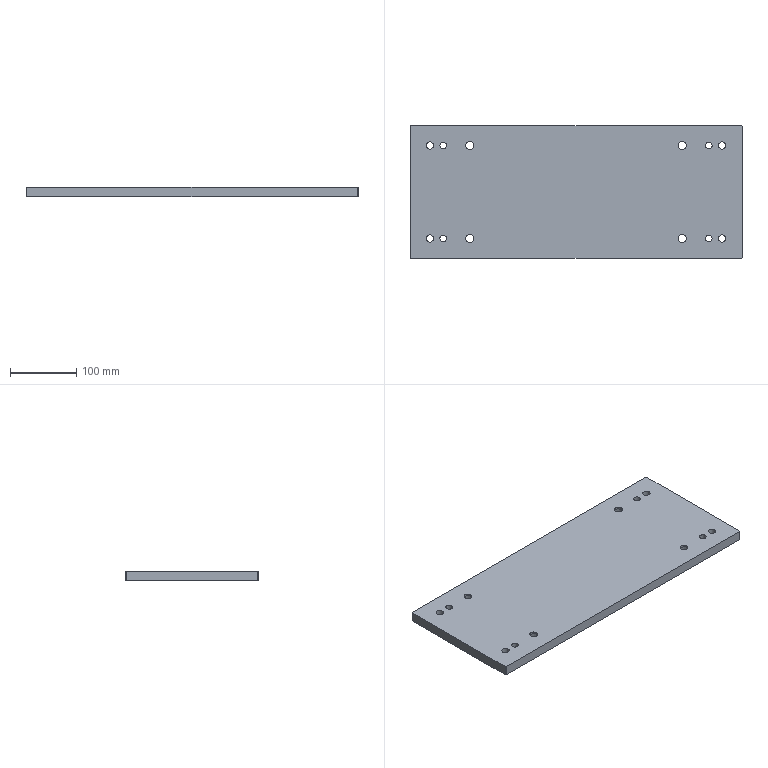Part | NX | features BREP 1 | 1 solid | 30 faces | box 500 x 200 x 15 mm | volume 1469857 mm3 | cylinder 16 | plane 14 | commonest cylinder face diameters 10.1 x4 11 x4 12 x4 22 x4
STEP:
#1=CARTESIAN_POINT('',(-250.,-99.,67.));
#2=VERTEX_POINT('',#1);
#3=CARTESIAN_POINT('',(-250.,99.,67.));
#4=VERTEX_POINT('',#3);
#5=CARTESIAN_POINT('',(-250.,-100.,67.));
#6=DIRECTION('',(0.,1.,0.));
#7=VECTOR('',#6,1000.);
#8=LINE('',#5,#7);
#9=EDGE_CURVE('',#2,#4,#8,.T.);
#10=ORIENTED_EDGE('',*,*,#9,.T.);
#11=CARTESIAN_POINT('',(-250.,99.,52.));
#12=VERTEX_POINT('',#11);
#13=CARTESIAN_POINT('',(-250.,99.,52.));
#14=DIRECTION('',(0.,0.,-1.));
#15=VECTOR('',#14,1000.);
#16=LINE('',#13,#15);
#17=EDGE_CURVE('',#4,#12,#16,.T.);
#18=ORIENTED_EDGE('',*,*,#17,.T.);
#19=CARTESIAN_POINT('',(-250.,-99.,52.));
#20=VERTEX_POINT('',#19);
#21=CARTESIAN_POINT('',(-250.,-100.,52.));
#22=DIRECTION('',(0.,1.,0.));
#23=VECTOR('',#22,1000.);
#24=LINE('',#21,#23);
#25=EDGE_CURVE('',#20,#12,#24,.T.);
#26=ORIENTED_EDGE('',*,*,#25,.F.);
#27=CARTESIAN_POINT('',(-250.,-99.,52.));
#28=DIRECTION('',(0.,0.,1.));
#29=VECTOR('',#28,1000.);
#30=LINE('',#27,#29);
#31=EDGE_CURVE('',#20,#2,#30,.T.);
#32=ORIENTED_EDGE('',*,*,#31,.T.);
#33=EDGE_LOOP('',(#10,#18,#26,#32));
#34=FACE_BOUND('',#33,.T.);
#35=CARTESIAN_POINT('',(-250.,-100.,52.));
#36=DIRECTION('',(1.,0.,0.));
#37=DIRECTION('',(0.,0.,1.));
#38=AXIS2_PLACEMENT_3D('',#35,#36,#37);
#39=PLANE('',#38);
#40=ADVANCED_FACE('',(#34),#39,.F.);
#41=CARTESIAN_POINT('',(-249.,100.,52.));
#42=VERTEX_POINT('',#41);
#43=CARTESIAN_POINT('',(249.,100.,52.));
#44=VERTEX_POINT('',#43);
#45=CARTESIAN_POINT('',(-250.,100.,52.));
#46=DIRECTION('',(1.,0.,0.));
#47=VECTOR('',#46,1000.);
#48=LINE('',#45,#47);
#49=EDGE_CURVE('',#42,#44,#48,.T.);
#50=ORIENTED_EDGE('',*,*,#49,.F.);
#51=CARTESIAN_POINT('',(-249.,100.,67.));
#52=VERTEX_POINT('',#51);
#53=CARTESIAN_POINT('',(-249.,100.,52.));
#54=DIRECTION('',(0.,0.,1.));
#55=VECTOR('',#54,1000.);
#56=LINE('',#53,#55);
#57=EDGE_CURVE('',#42,#52,#56,.T.);
#58=ORIENTED_EDGE('',*,*,#57,.T.);
#59=CARTESIAN_POINT('',(249.,100.,67.));
#60=VERTEX_POINT('',#59);
#61=CARTESIAN_POINT('',(-250.,100.,67.));
#62=DIRECTION('',(1.,0.,0.));
#63=VECTOR('',#62,1000.);
#64=LINE('',#61,#63);
#65=EDGE_CURVE('',#52,#60,#64,.T.);
#66=ORIENTED_EDGE('',*,*,#65,.T.);
#67=CARTESIAN_POINT('',(249.,100.,52.));
#68=DIRECTION('',(0.,0.,-1.));
#69=VECTOR('',#68,1000.);
#70=LINE('',#67,#69);
#71=EDGE_CURVE('',#60,#44,#70,.T.);
#72=ORIENTED_EDGE('',*,*,#71,.T.);
#73=EDGE_LOOP('',(#50,#58,#66,#72));
#74=FACE_BOUND('',#73,.T.);
#75=CARTESIAN_POINT('',(-250.,100.,52.));
#76=DIRECTION('',(0.,-1.,0.));
#77=DIRECTION('',(0.,0.,1.));
#78=AXIS2_PLACEMENT_3D('',#75,#76,#77);
#79=PLANE('',#78);
#80=ADVANCED_FACE('',(#74),#79,.F.);
#81=CARTESIAN_POINT('',(250.,99.,52.));
#82=VERTEX_POINT('',#81);
#83=CARTESIAN_POINT('',(250.,-99.,52.));
#84=VERTEX_POINT('',#83);
#85=CARTESIAN_POINT('',(250.,100.,52.));
#86=DIRECTION('',(0.,-1.,0.));
#87=VECTOR('',#86,1000.);
#88=LINE('',#85,#87);
#89=EDGE_CURVE('',#82,#84,#88,.T.);
#90=ORIENTED_EDGE('',*,*,#89,.F.);
#91=CARTESIAN_POINT('',(250.,99.,67.));
#92=VERTEX_POINT('',#91);
#93=CARTESIAN_POINT('',(250.,99.,52.));
#94=DIRECTION('',(0.,0.,1.));
#95=VECTOR('',#94,1000.);
#96=LINE('',#93,#95);
#97=EDGE_CURVE('',#82,#92,#96,.T.);
#98=ORIENTED_EDGE('',*,*,#97,.T.);
#99=CARTESIAN_POINT('',(250.,-99.,67.));
#100=VERTEX_POINT('',#99);
#101=CARTESIAN_POINT('',(250.,100.,67.));
#102=DIRECTION('',(0.,-1.,0.));
#103=VECTOR('',#102,1000.);
#104=LINE('',#101,#103);
#105=EDGE_CURVE('',#92,#100,#104,.T.);
#106=ORIENTED_EDGE('',*,*,#105,.T.);
#107=CARTESIAN_POINT('',(250.,-99.,52.));
#108=DIRECTION('',(0.,0.,-1.));
#109=VECTOR('',#108,1000.);
#110=LINE('',#107,#109);
#111=EDGE_CURVE('',#100,#84,#110,.T.);
#112=ORIENTED_EDGE('',*,*,#111,.T.);
#113=EDGE_LOOP('',(#90,#98,#106,#112));
#114=FACE_BOUND('',#113,.T.);
#115=CARTESIAN_POINT('',(250.,100.,52.));
#116=DIRECTION('',(-1.,0.,0.));
#117=DIRECTION('',(0.,0.,-1.));
#118=AXIS2_PLACEMENT_3D('',#115,#116,#117);
#119=PLANE('',#118);
#120=ADVANCED_FACE('',(#114),#119,.F.);
#121=CARTESIAN_POINT('',(249.,-100.,52.));
#122=VERTEX_POINT('',#121);
#123=CARTESIAN_POINT('',(-249.,-100.,52.));
#124=VERTEX_POINT('',#123);
#125=CARTESIAN_POINT('',(250.,-100.,52.));
#126=DIRECTION('',(-1.,0.,0.));
#127=VECTOR('',#126,1000.);
#128=LINE('',#125,#127);
#129=EDGE_CURVE('',#122,#124,#128,.T.);
#130=ORIENTED_EDGE('',*,*,#129,.F.);
#131=CARTESIAN_POINT('',(249.,-100.,67.));
#132=VERTEX_POINT('',#131);
#133=CARTESIAN_POINT('',(249.,-100.,52.));
#134=DIRECTION('',(0.,0.,1.));
#135=VECTOR('',#134,1000.);
#136=LINE('',#133,#135);
#137=EDGE_CURVE('',#122,#132,#136,.T.);
#138=ORIENTED_EDGE('',*,*,#137,.T.);
#139=CARTESIAN_POINT('',(-249.,-100.,67.));
#140=VERTEX_POINT('',#139);
#141=CARTESIAN_POINT('',(250.,-100.,67.));
#142=DIRECTION('',(-1.,0.,0.));
#143=VECTOR('',#142,1000.);
#144=LINE('',#141,#143);
#145=EDGE_CURVE('',#132,#140,#144,.T.);
#146=ORIENTED_EDGE('',*,*,#145,.T.);
#147=CARTESIAN_POINT('',(-249.,-100.,52.));
#148=DIRECTION('',(0.,0.,-1.));
#149=VECTOR('',#148,1000.);
#150=LINE('',#147,#149);
#151=EDGE_CURVE('',#140,#124,#150,.T.);
#152=ORIENTED_EDGE('',*,*,#151,.T.);
#153=EDGE_LOOP('',(#130,#138,#146,#152));
#154=FACE_BOUND('',#153,.T.);
#155=CARTESIAN_POINT('',(250.,-100.,52.));
#156=DIRECTION('',(0.,1.,0.));
#157=DIRECTION('',(1.,0.,0.));
#158=AXIS2_PLACEMENT_3D('',#155,#156,#157);
#159=PLANE('',#158);
#160=ADVANCED_FACE('',(#154),#159,.F.);
#161=CARTESIAN_POINT('',(-171.,70.,52.));
#162=VERTEX_POINT('',#161);
#163=CARTESIAN_POINT('',(-160.,70.,52.));
#164=DIRECTION('',(0.,0.,1.));
#165=DIRECTION('',(-1.,0.,0.));
#166=AXIS2_PLACEMENT_3D('',#163,#164,#165);
#167=CIRCLE('',#166,11.);
#168=EDGE_CURVE('',#162,#162,#167,.T.);
#169=ORIENTED_EDGE('',*,*,#168,.T.);
#170=EDGE_LOOP('',(#169));
#171=FACE_BOUND('',#170,.T.);
#172=CARTESIAN_POINT('',(-171.,-70.,52.));
#173=VERTEX_POINT('',#172);
#174=CARTESIAN_POINT('',(-160.,-70.,52.));
#175=DIRECTION('',(0.,0.,1.));
#176=DIRECTION('',(-1.,0.,0.));
#177=AXIS2_PLACEMENT_3D('',#174,#175,#176);
#178=CIRCLE('',#177,11.);
#179=EDGE_CURVE('',#173,#173,#178,.T.);
#180=ORIENTED_EDGE('',*,*,#179,.T.);
#181=EDGE_LOOP('',(#180));
#182=FACE_BOUND('',#181,.T.);
#183=CARTESIAN_POINT('',(149.,70.,52.));
#184=VERTEX_POINT('',#183);
#185=CARTESIAN_POINT('',(160.,70.,52.));
#186=DIRECTION('',(0.,0.,1.));
#187=DIRECTION('',(-1.,0.,0.));
#188=AXIS2_PLACEMENT_3D('',#185,#186,#187);
#189=CIRCLE('',#188,11.);
#190=EDGE_CURVE('',#184,#184,#189,.T.);
#191=ORIENTED_EDGE('',*,*,#190,.T.);
#192=EDGE_LOOP('',(#191));
#193=FACE_BOUND('',#192,.T.);
#194=CARTESIAN_POINT('',(149.,-70.,52.));
#195=VERTEX_POINT('',#194);
#196=CARTESIAN_POINT('',(160.,-70.,52.));
#197=DIRECTION('',(0.,0.,1.));
#198=DIRECTION('',(-1.,0.,0.));
#199=AXIS2_PLACEMENT_3D('',#196,#197,#198);
#200=CIRCLE('',#199,11.);
#201=EDGE_CURVE('',#195,#195,#200,.T.);
#202=ORIENTED_EDGE('',*,*,#201,.T.);
#203=EDGE_LOOP('',(#202));
#204=FACE_BOUND('',#203,.T.);
#205=CARTESIAN_POINT('',(195.335,71.934,52.));
#206=VERTEX_POINT('',#205);
#207=CARTESIAN_POINT('',(200.,70.,52.));
#208=DIRECTION('',(0.,0.,-1.));
#209=DIRECTION('',(-0.9237,0.383,0.));
#210=AXIS2_PLACEMENT_3D('',#207,#208,#209);
#211=CIRCLE('',#210,5.05);
#212=EDGE_CURVE('',#206,#206,#211,.T.);
#213=ORIENTED_EDGE('',*,*,#212,.F.);
#214=EDGE_LOOP('',(#213));
#215=FACE_BOUND('',#214,.T.);
#216=CARTESIAN_POINT('',(195.335,-68.066,52.));
#217=VERTEX_POINT('',#216);
#218=CARTESIAN_POINT('',(200.,-70.,52.));
#219=DIRECTION('',(0.,0.,-1.));
#220=DIRECTION('',(-0.9237,0.383,0.));
#221=AXIS2_PLACEMENT_3D('',#218,#219,#220);
#222=CIRCLE('',#221,5.05);
#223=EDGE_CURVE('',#217,#217,#222,.T.);
#224=ORIENTED_EDGE('',*,*,#223,.F.);
#225=EDGE_LOOP('',(#224));
#226=FACE_BOUND('',#225,.T.);
#227=CARTESIAN_POINT('',(-204.665,71.934,52.));
#228=VERTEX_POINT('',#227);
#229=CARTESIAN_POINT('',(-200.,70.,52.));
#230=DIRECTION('',(0.,0.,-1.));
#231=DIRECTION('',(-0.9237,0.383,0.));
#232=AXIS2_PLACEMENT_3D('',#229,#230,#231);
#233=CIRCLE('',#232,5.05);
#234=EDGE_CURVE('',#228,#228,#233,.T.);
#235=ORIENTED_EDGE('',*,*,#234,.F.);
#236=EDGE_LOOP('',(#235));
#237=FACE_BOUND('',#236,.T.);
#238=CARTESIAN_POINT('',(-204.665,-68.066,52.));
#239=VERTEX_POINT('',#238);
#240=CARTESIAN_POINT('',(-200.,-70.,52.));
#241=DIRECTION('',(0.,0.,-1.));
#242=DIRECTION('',(-0.9237,0.383,0.));
#243=AXIS2_PLACEMENT_3D('',#240,#241,#242);
#244=CIRCLE('',#243,5.05);
#245=EDGE_CURVE('',#239,#239,#244,.T.);
#246=ORIENTED_EDGE('',*,*,#245,.F.);
#247=EDGE_LOOP('',(#246));
#248=FACE_BOUND('',#247,.T.);
#249=CARTESIAN_POINT('',(214.5,-70.,52.));
#250=VERTEX_POINT('',#249);
#251=CARTESIAN_POINT('',(220.,-70.,52.));
#252=DIRECTION('',(0.,0.,-1.));
#253=DIRECTION('',(-1.,0.,0.));
#254=AXIS2_PLACEMENT_3D('',#251,#252,#253);
#255=CIRCLE('',#254,5.5);
#256=EDGE_CURVE('',#250,#250,#255,.T.);
#257=ORIENTED_EDGE('',*,*,#256,.F.);
#258=EDGE_LOOP('',(#257));
#259=FACE_BOUND('',#258,.T.);
#260=CARTESIAN_POINT('',(-225.5,70.,52.));
#261=VERTEX_POINT('',#260);
#262=CARTESIAN_POINT('',(-220.,70.,52.));
#263=DIRECTION('',(0.,0.,-1.));
#264=DIRECTION('',(-1.,0.,0.));
#265=AXIS2_PLACEMENT_3D('',#262,#263,#264);
#266=CIRCLE('',#265,5.5);
#267=EDGE_CURVE('',#261,#261,#266,.T.);
#268=ORIENTED_EDGE('',*,*,#267,.F.);
#269=EDGE_LOOP('',(#268));
#270=FACE_BOUND('',#269,.T.);
#271=CARTESIAN_POINT('',(-225.5,-70.,52.));
#272=VERTEX_POINT('',#271);
#273=CARTESIAN_POINT('',(-220.,-70.,52.));
#274=DIRECTION('',(0.,0.,-1.));
#275=DIRECTION('',(-1.,0.,0.));
#276=AXIS2_PLACEMENT_3D('',#273,#274,#275);
#277=CIRCLE('',#276,5.5);
#278=EDGE_CURVE('',#272,#272,#277,.T.);
#279=ORIENTED_EDGE('',*,*,#278,.F.);
#280=EDGE_LOOP('',(#279));
#281=FACE_BOUND('',#280,.T.);
#282=CARTESIAN_POINT('',(214.5,70.,52.));
#283=VERTEX_POINT('',#282);
#284=CARTESIAN_POINT('',(220.,70.,52.));
#285=DIRECTION('',(0.,0.,-1.));
#286=DIRECTION('',(-1.,0.,0.));
#287=AXIS2_PLACEMENT_3D('',#284,#285,#286);
#288=CIRCLE('',#287,5.5);
#289=EDGE_CURVE('',#283,#283,#288,.T.);
#290=ORIENTED_EDGE('',*,*,#289,.F.);
#291=EDGE_LOOP('',(#290));
#292=FACE_BOUND('',#291,.T.);
#293=ORIENTED_EDGE('',*,*,#25,.T.);
#294=CARTESIAN_POINT('',(-249.5,99.5,52.));
#295=DIRECTION('',(0.7071,0.7071,0.));
#296=VECTOR('',#295,1000.);
#297=LINE('',#294,#296);
#298=EDGE_CURVE('',#12,#42,#297,.T.);
#299=ORIENTED_EDGE('',*,*,#298,.T.);
#300=ORIENTED_EDGE('',*,*,#49,.T.);
#301=CARTESIAN_POINT('',(-0.5,349.5,52.));
#302=DIRECTION('',(0.7071,-0.7071,0.));
#303=VECTOR('',#302,1000.);
#304=LINE('',#301,#303);
#305=EDGE_CURVE('',#44,#82,#304,.T.);
#306=ORIENTED_EDGE('',*,*,#305,.T.);
#307=ORIENTED_EDGE('',*,*,#89,.T.);
#308=CARTESIAN_POINT('',(99.5,-249.5,52.));
#309=DIRECTION('',(-0.7071,-0.7071,0.));
#310=VECTOR('',#309,1000.);
#311=LINE('',#308,#310);
#312=EDGE_CURVE('',#84,#122,#311,.T.);
#313=ORIENTED_EDGE('',*,*,#312,.T.);
#314=ORIENTED_EDGE('',*,*,#129,.T.);
#315=CARTESIAN_POINT('',(-349.5,0.5,52.));
#316=DIRECTION('',(-0.7071,0.7071,0.));
#317=VECTOR('',#316,1000.);
#318=LINE('',#315,#317);
#319=EDGE_CURVE('',#124,#20,#318,.T.);
#320=ORIENTED_EDGE('',*,*,#319,.T.);
#321=EDGE_LOOP('',(#293,#299,#300,#306,#307,#313,#314,#320));
#322=FACE_BOUND('',#321,.T.);
#323=CARTESIAN_POINT('',(-250.,100.,52.));
#324=DIRECTION('',(0.,0.,-1.));
#325=DIRECTION('',(1.,0.,0.));
#326=AXIS2_PLACEMENT_3D('',#323,#324,#325);
#327=PLANE('',#326);
#328=ADVANCED_FACE('',(#171,#182,#193,#204,#215,#226,#237,#248,#259,#270,#281,#292,#322),#327,.T.);
#329=CARTESIAN_POINT('',(195.335,71.934,67.));
#330=VERTEX_POINT('',#329);
#331=CARTESIAN_POINT('',(200.,70.,67.));
#332=DIRECTION('',(0.,0.,-1.));
#333=DIRECTION('',(-0.9237,0.383,0.));
#334=AXIS2_PLACEMENT_3D('',#331,#332,#333);
#335=CIRCLE('',#334,5.05);
#336=EDGE_CURVE('',#330,#330,#335,.T.);
#337=ORIENTED_EDGE('',*,*,#336,.T.);
#338=EDGE_LOOP('',(#337));
#339=FACE_BOUND('',#338,.T.);
#340=CARTESIAN_POINT('',(195.335,-68.066,67.));
#341=VERTEX_POINT('',#340);
#342=CARTESIAN_POINT('',(200.,-70.,67.));
#343=DIRECTION('',(0.,0.,-1.));
#344=DIRECTION('',(-0.9237,0.383,0.));
#345=AXIS2_PLACEMENT_3D('',#342,#343,#344);
#346=CIRCLE('',#345,5.05);
#347=EDGE_CURVE('',#341,#341,#346,.T.);
#348=ORIENTED_EDGE('',*,*,#347,.T.);
#349=EDGE_LOOP('',(#348));
#350=FACE_BOUND('',#349,.T.);
#351=CARTESIAN_POINT('',(-204.665,71.934,67.));
#352=VERTEX_POINT('',#351);
#353=CARTESIAN_POINT('',(-200.,70.,67.));
#354=DIRECTION('',(0.,0.,-1.));
#355=DIRECTION('',(-0.9237,0.383,0.));
#356=AXIS2_PLACEMENT_3D('',#353,#354,#355);
#357=CIRCLE('',#356,5.05);
#358=EDGE_CURVE('',#352,#352,#357,.T.);
#359=ORIENTED_EDGE('',*,*,#358,.T.);
#360=EDGE_LOOP('',(#359));
#361=FACE_BOUND('',#360,.T.);
#362=CARTESIAN_POINT('',(-204.665,-68.066,67.));
#363=VERTEX_POINT('',#362);
#364=CARTESIAN_POINT('',(-200.,-70.,67.));
#365=DIRECTION('',(0.,0.,-1.));
#366=DIRECTION('',(-0.9237,0.383,0.));
#367=AXIS2_PLACEMENT_3D('',#364,#365,#366);
#368=CIRCLE('',#367,5.05);
#369=EDGE_CURVE('',#363,#363,#368,.T.);
#370=ORIENTED_EDGE('',*,*,#369,.T.);
#371=EDGE_LOOP('',(#370));
#372=FACE_BOUND('',#371,.T.);
#373=CARTESIAN_POINT('',(214.5,-70.,67.));
#374=VERTEX_POINT('',#373);
#375=CARTESIAN_POINT('',(220.,-70.,67.));
#376=DIRECTION('',(0.,0.,-1.));
#377=DIRECTION('',(-1.,0.,0.));
#378=AXIS2_PLACEMENT_3D('',#375,#376,#377);
#379=CIRCLE('',#378,5.5);
#380=EDGE_CURVE('',#374,#374,#379,.T.);
#381=ORIENTED_EDGE('',*,*,#380,.T.);
#382=EDGE_LOOP('',(#381));
#383=FACE_BOUND('',#382,.T.);
#384=CARTESIAN_POINT('',(-225.5,70.,67.));
#385=VERTEX_POINT('',#384);
#386=CARTESIAN_POINT('',(-220.,70.,67.));
#387=DIRECTION('',(0.,0.,-1.));
#388=DIRECTION('',(-1.,0.,0.));
#389=AXIS2_PLACEMENT_3D('',#386,#387,#388);
#390=CIRCLE('',#389,5.5);
#391=EDGE_CURVE('',#385,#385,#390,.T.);
#392=ORIENTED_EDGE('',*,*,#391,.T.);
#393=EDGE_LOOP('',(#392));
#394=FACE_BOUND('',#393,.T.);
#395=CARTESIAN_POINT('',(-225.5,-70.,67.));
#396=VERTEX_POINT('',#395);
#397=CARTESIAN_POINT('',(-220.,-70.,67.));
#398=DIRECTION('',(0.,0.,-1.));
#399=DIRECTION('',(-1.,0.,0.));
#400=AXIS2_PLACEMENT_3D('',#397,#398,#399);
#401=CIRCLE('',#400,5.5);
#402=EDGE_CURVE('',#396,#396,#401,.T.);
#403=ORIENTED_EDGE('',*,*,#402,.T.);
#404=EDGE_LOOP('',(#403));
#405=FACE_BOUND('',#404,.T.);
#406=CARTESIAN_POINT('',(214.5,70.,67.));
#407=VERTEX_POINT('',#406);
#408=CARTESIAN_POINT('',(220.,70.,67.));
#409=DIRECTION('',(0.,0.,-1.));
#410=DIRECTION('',(-1.,0.,0.));
#411=AXIS2_PLACEMENT_3D('',#408,#409,#410);
#412=CIRCLE('',#411,5.5);
#413=EDGE_CURVE('',#407,#407,#412,.T.);
#414=ORIENTED_EDGE('',*,*,#413,.T.);
#415=EDGE_LOOP('',(#414));
#416=FACE_BOUND('',#415,.T.);
#417=CARTESIAN_POINT('',(154.,-70.,67.));
#418=VERTEX_POINT('',#417);
#419=CARTESIAN_POINT('',(160.,-70.,67.));
#420=DIRECTION('',(0.,0.,1.));
#421=DIRECTION('',(-1.,0.,0.));
#422=AXIS2_PLACEMENT_3D('',#419,#420,#421);
#423=CIRCLE('',#422,6.);
#424=EDGE_CURVE('',#418,#418,#423,.T.);
#425=ORIENTED_EDGE('',*,*,#424,.F.);
#426=EDGE_LOOP('',(#425));
#427=FACE_BOUND('',#426,.T.);
#428=CARTESIAN_POINT('',(-166.,70.,67.));
#429=VERTEX_POINT('',#428);
#430=CARTESIAN_POINT('',(-160.,70.,67.));
#431=DIRECTION('',(0.,0.,1.));
#432=DIRECTION('',(-1.,0.,0.));
#433=AXIS2_PLACEMENT_3D('',#430,#431,#432);
#434=CIRCLE('',#433,6.);
#435=EDGE_CURVE('',#429,#429,#434,.T.);
#436=ORIENTED_EDGE('',*,*,#435,.F.);
#437=EDGE_LOOP('',(#436));
#438=FACE_BOUND('',#437,.T.);
#439=CARTESIAN_POINT('',(-166.,-70.,67.));
#440=VERTEX_POINT('',#439);
#441=CARTESIAN_POINT('',(-160.,-70.,67.));
#442=DIRECTION('',(0.,0.,1.));
#443=DIRECTION('',(-1.,0.,0.));
#444=AXIS2_PLACEMENT_3D('',#441,#442,#443);
#445=CIRCLE('',#444,6.);
#446=EDGE_CURVE('',#440,#440,#445,.T.);
#447=ORIENTED_EDGE('',*,*,#446,.F.);
#448=EDGE_LOOP('',(#447));
#449=FACE_BOUND('',#448,.T.);
#450=CARTESIAN_POINT('',(154.,70.,67.));
#451=VERTEX_POINT('',#450);
#452=CARTESIAN_POINT('',(160.,70.,67.));
#453=DIRECTION('',(0.,0.,1.));
#454=DIRECTION('',(-1.,0.,0.));
#455=AXIS2_PLACEMENT_3D('',#452,#453,#454);
#456=CIRCLE('',#455,6.);
#457=EDGE_CURVE('',#451,#451,#456,.T.);
#458=ORIENTED_EDGE('',*,*,#457,.F.);
#459=EDGE_LOOP('',(#458));
#460=FACE_BOUND('',#459,.T.);
#461=ORIENTED_EDGE('',*,*,#65,.F.);
#462=CARTESIAN_POINT('',(-249.,100.,67.));
#463=DIRECTION('',(-0.7071,-0.7071,0.));
#464=VECTOR('',#463,1000.);
#465=LINE('',#462,#464);
#466=EDGE_CURVE('',#52,#4,#465,.T.);
#467=ORIENTED_EDGE('',*,*,#466,.T.);
#468=ORIENTED_EDGE('',*,*,#9,.F.);
#469=CARTESIAN_POINT('',(-250.,-99.,67.));
#470=DIRECTION('',(0.7071,-0.7071,0.));
#471=VECTOR('',#470,1000.);
#472=LINE('',#469,#471);
#473=EDGE_CURVE('',#2,#140,#472,.T.);
#474=ORIENTED_EDGE('',*,*,#473,.T.);
#475=ORIENTED_EDGE('',*,*,#145,.F.);
#476=CARTESIAN_POINT('',(249.,-100.,67.));
#477=DIRECTION('',(0.7071,0.7071,0.));
#478=VECTOR('',#477,1000.);
#479=LINE('',#476,#478);
#480=EDGE_CURVE('',#132,#100,#479,.T.);
#481=ORIENTED_EDGE('',*,*,#480,.T.);
#482=ORIENTED_EDGE('',*,*,#105,.F.);
#483=CARTESIAN_POINT('',(250.,99.,67.));
#484=DIRECTION('',(-0.7071,0.7071,0.));
#485=VECTOR('',#484,1000.);
#486=LINE('',#483,#485);
#487=EDGE_CURVE('',#92,#60,#486,.T.);
#488=ORIENTED_EDGE('',*,*,#487,.T.);
#489=EDGE_LOOP('',(#461,#467,#468,#474,#475,#481,#482,#488));
#490=FACE_BOUND('',#489,.T.);
#491=CARTESIAN_POINT('',(-250.,100.,67.));
#492=DIRECTION('',(0.,0.,-1.));
#493=DIRECTION('',(1.,0.,0.));
#494=AXIS2_PLACEMENT_3D('',#491,#492,#493);
#495=PLANE('',#494);
#496=ADVANCED_FACE('',(#339,#350,#361,#372,#383,#394,#405,#416,#427,#438,#449,#460,#490),#495,.F.);
#497=ORIENTED_EDGE('',*,*,#298,.F.);
#498=ORIENTED_EDGE('',*,*,#17,.F.);
#499=ORIENTED_EDGE('',*,*,#466,.F.);
#500=ORIENTED_EDGE('',*,*,#57,.F.);
#501=EDGE_LOOP('',(#497,#498,#499,#500));
#502=FACE_BOUND('',#501,.T.);
#503=CARTESIAN_POINT('',(-249.,100.,52.));
#504=DIRECTION('',(0.7071,-0.7071,0.));
#505=DIRECTION('',(-0.7071,-0.7071,0.));
#506=AXIS2_PLACEMENT_3D('',#503,#504,#505);
#507=PLANE('',#506);
#508=ADVANCED_FACE('',(#502),#507,.F.);
#509=ORIENTED_EDGE('',*,*,#305,.F.);
#510=ORIENTED_EDGE('',*,*,#71,.F.);
#511=ORIENTED_EDGE('',*,*,#487,.F.);
#512=ORIENTED_EDGE('',*,*,#97,.F.);
#513=EDGE_LOOP('',(#509,#510,#511,#512));
#514=FACE_BOUND('',#513,.T.);
#515=CARTESIAN_POINT('',(250.,99.,52.));
#516=DIRECTION('',(-0.7071,-0.7071,0.));
#517=DIRECTION('',(-0.7071,0.7071,0.));
#518=AXIS2_PLACEMENT_3D('',#515,#516,#517);
#519=PLANE('',#518);
#520=ADVANCED_FACE('',(#514),#519,.F.);
#521=ORIENTED_EDGE('',*,*,#312,.F.);
#522=ORIENTED_EDGE('',*,*,#111,.F.);
#523=ORIENTED_EDGE('',*,*,#480,.F.);
#524=ORIENTED_EDGE('',*,*,#137,.F.);
#525=EDGE_LOOP('',(#521,#522,#523,#524));
#526=FACE_BOUND('',#525,.T.);
#527=CARTESIAN_POINT('',(249.,-100.,52.));
#528=DIRECTION('',(-0.7071,0.7071,0.));
#529=DIRECTION('',(0.7071,0.7071,0.));
#530=AXIS2_PLACEMENT_3D('',#527,#528,#529);
#531=PLANE('',#530);
#532=ADVANCED_FACE('',(#526),#531,.F.);
#533=ORIENTED_EDGE('',*,*,#319,.F.);
#534=ORIENTED_EDGE('',*,*,#151,.F.);
#535=ORIENTED_EDGE('',*,*,#473,.F.);
#536=ORIENTED_EDGE('',*,*,#31,.F.);
#537=EDGE_LOOP('',(#533,#534,#535,#536));
#538=FACE_BOUND('',#537,.T.);
#539=CARTESIAN_POINT('',(-250.,-99.,52.));
#540=DIRECTION('',(0.7071,0.7071,0.));
#541=DIRECTION('',(0.7071,-0.7071,0.));
#542=AXIS2_PLACEMENT_3D('',#539,#540,#541);
#543=PLANE('',#542);
#544=ADVANCED_FACE('',(#538),#543,.F.);
#545=CARTESIAN_POINT('',(166.,70.,64.));
#546=VERTEX_POINT('',#545);
#547=CARTESIAN_POINT('',(160.,70.,64.));
#548=DIRECTION('',(0.,0.,1.));
#549=DIRECTION('',(1.,0.,0.));
#550=AXIS2_PLACEMENT_3D('',#547,#548,#549);
#551=CIRCLE('',#550,6.);
#552=EDGE_CURVE('',#546,#546,#551,.T.);
#553=ORIENTED_EDGE('',*,*,#552,.F.);
#554=EDGE_LOOP('',(#553));
#555=FACE_BOUND('',#554,.T.);
#556=ORIENTED_EDGE('',*,*,#457,.T.);
#557=EDGE_LOOP('',(#556));
#558=FACE_BOUND('',#557,.T.);
#559=CARTESIAN_POINT('',(160.,70.,75.));
#560=DIRECTION('',(0.,0.,-1.));
#561=DIRECTION('',(1.,0.,0.));
#562=AXIS2_PLACEMENT_3D('',#559,#560,#561);
#563=CYLINDRICAL_SURFACE('',#562,6.);
#564=ADVANCED_FACE('',(#555,#558),#563,.F.);
#565=CARTESIAN_POINT('',(-154.,-70.,64.));
#566=VERTEX_POINT('',#565);
#567=CARTESIAN_POINT('',(-160.,-70.,64.));
#568=DIRECTION('',(0.,0.,1.));
#569=DIRECTION('',(1.,0.,0.));
#570=AXIS2_PLACEMENT_3D('',#567,#568,#569);
#571=CIRCLE('',#570,6.);
#572=EDGE_CURVE('',#566,#566,#571,.T.);
#573=ORIENTED_EDGE('',*,*,#572,.F.);
#574=EDGE_LOOP('',(#573));
#575=FACE_BOUND('',#574,.T.);
#576=ORIENTED_EDGE('',*,*,#446,.T.);
#577=EDGE_LOOP('',(#576));
#578=FACE_BOUND('',#577,.T.);
#579=CARTESIAN_POINT('',(-160.,-70.,75.));
#580=DIRECTION('',(0.,0.,-1.));
#581=DIRECTION('',(1.,0.,0.));
#582=AXIS2_PLACEMENT_3D('',#579,#580,#581);
#583=CYLINDRICAL_SURFACE('',#582,6.);
#584=ADVANCED_FACE('',(#575,#578),#583,.F.);
#585=CARTESIAN_POINT('',(-154.,70.,64.));
#586=VERTEX_POINT('',#585);
#587=CARTESIAN_POINT('',(-160.,70.,64.));
#588=DIRECTION('',(0.,0.,1.));
#589=DIRECTION('',(1.,0.,0.));
#590=AXIS2_PLACEMENT_3D('',#587,#588,#589);
#591=CIRCLE('',#590,6.);
#592=EDGE_CURVE('',#586,#586,#591,.T.);
#593=ORIENTED_EDGE('',*,*,#592,.F.);
#594=EDGE_LOOP('',(#593));
#595=FACE_BOUND('',#594,.T.);
#596=ORIENTED_EDGE('',*,*,#435,.T.);
#597=EDGE_LOOP('',(#596));
#598=FACE_BOUND('',#597,.T.);
#599=CARTESIAN_POINT('',(-160.,70.,75.));
#600=DIRECTION('',(0.,0.,-1.));
#601=DIRECTION('',(1.,0.,0.));
#602=AXIS2_PLACEMENT_3D('',#599,#600,#601);
#603=CYLINDRICAL_SURFACE('',#602,6.);
#604=ADVANCED_FACE('',(#595,#598),#603,.F.);
#605=CARTESIAN_POINT('',(166.,-70.,64.));
#606=VERTEX_POINT('',#605);
#607=CARTESIAN_POINT('',(160.,-70.,64.));
#608=DIRECTION('',(0.,0.,1.));
#609=DIRECTION('',(1.,0.,0.));
#610=AXIS2_PLACEMENT_3D('',#607,#608,#609);
#611=CIRCLE('',#610,6.);
#612=EDGE_CURVE('',#606,#606,#611,.T.);
#613=ORIENTED_EDGE('',*,*,#612,.F.);
#614=EDGE_LOOP('',(#613));
#615=FACE_BOUND('',#614,.T.);
#616=ORIENTED_EDGE('',*,*,#424,.T.);
#617=EDGE_LOOP('',(#616));
#618=FACE_BOUND('',#617,.T.);
#619=CARTESIAN_POINT('',(160.,-70.,75.));
#620=DIRECTION('',(0.,0.,-1.));
#621=DIRECTION('',(1.,0.,0.));
#622=AXIS2_PLACEMENT_3D('',#619,#620,#621);
#623=CYLINDRICAL_SURFACE('',#622,6.);
#624=ADVANCED_FACE('',(#615,#618),#623,.F.);
#625=ORIENTED_EDGE('',*,*,#289,.T.);
#626=EDGE_LOOP('',(#625));
#627=FACE_BOUND('',#626,.T.);
#628=ORIENTED_EDGE('',*,*,#413,.F.);
#629=EDGE_LOOP('',(#628));
#630=FACE_BOUND('',#629,.T.);
#631=CARTESIAN_POINT('',(220.,70.,103.));
#632=DIRECTION('',(0.,0.,-1.));
#633=DIRECTION('',(1.,0.,0.));
#634=AXIS2_PLACEMENT_3D('',#631,#632,#633);
#635=CYLINDRICAL_SURFACE('',#634,5.5);
#636=ADVANCED_FACE('',(#627,#630),#635,.F.);
#637=ORIENTED_EDGE('',*,*,#278,.T.);
#638=EDGE_LOOP('',(#637));
#639=FACE_BOUND('',#638,.T.);
#640=ORIENTED_EDGE('',*,*,#402,.F.);
#641=EDGE_LOOP('',(#640));
#642=FACE_BOUND('',#641,.T.);
#643=CARTESIAN_POINT('',(-220.,-70.,103.));
#644=DIRECTION('',(0.,0.,-1.));
#645=DIRECTION('',(1.,0.,0.));
#646=AXIS2_PLACEMENT_3D('',#643,#644,#645);
#647=CYLINDRICAL_SURFACE('',#646,5.5);
#648=ADVANCED_FACE('',(#639,#642),#647,.F.);
#649=ORIENTED_EDGE('',*,*,#267,.T.);
#650=EDGE_LOOP('',(#649));
#651=FACE_BOUND('',#650,.T.);
#652=ORIENTED_EDGE('',*,*,#391,.F.);
#653=EDGE_LOOP('',(#652));
#654=FACE_BOUND('',#653,.T.);
#655=CARTESIAN_POINT('',(-220.,70.,103.));
#656=DIRECTION('',(0.,0.,-1.));
#657=DIRECTION('',(1.,0.,0.));
#658=AXIS2_PLACEMENT_3D('',#655,#656,#657);
#659=CYLINDRICAL_SURFACE('',#658,5.5);
#660=ADVANCED_FACE('',(#651,#654),#659,.F.);
#661=ORIENTED_EDGE('',*,*,#256,.T.);
#662=EDGE_LOOP('',(#661));
#663=FACE_BOUND('',#662,.T.);
#664=ORIENTED_EDGE('',*,*,#380,.F.);
#665=EDGE_LOOP('',(#664));
#666=FACE_BOUND('',#665,.T.);
#667=CARTESIAN_POINT('',(220.,-70.,103.));
#668=DIRECTION('',(0.,0.,-1.));
#669=DIRECTION('',(1.,0.,0.));
#670=AXIS2_PLACEMENT_3D('',#667,#668,#669);
#671=CYLINDRICAL_SURFACE('',#670,5.5);
#672=ADVANCED_FACE('',(#663,#666),#671,.F.);
#673=ORIENTED_EDGE('',*,*,#245,.T.);
#674=EDGE_LOOP('',(#673));
#675=FACE_BOUND('',#674,.T.);
#676=ORIENTED_EDGE('',*,*,#369,.F.);
#677=EDGE_LOOP('',(#676));
#678=FACE_BOUND('',#677,.T.);
#679=CARTESIAN_POINT('',(-200.,-70.,67.));
#680=DIRECTION('',(0.,0.,-1.));
#681=DIRECTION('',(0.9237,-0.383,0.));
#682=AXIS2_PLACEMENT_3D('',#679,#680,#681);
#683=CYLINDRICAL_SURFACE('',#682,5.05);
#684=ADVANCED_FACE('',(#675,#678),#683,.F.);
#685=ORIENTED_EDGE('',*,*,#234,.T.);
#686=EDGE_LOOP('',(#685));
#687=FACE_BOUND('',#686,.T.);
#688=ORIENTED_EDGE('',*,*,#358,.F.);
#689=EDGE_LOOP('',(#688));
#690=FACE_BOUND('',#689,.T.);
#691=CARTESIAN_POINT('',(-200.,70.,67.));
#692=DIRECTION('',(0.,0.,-1.));
#693=DIRECTION('',(0.9237,-0.383,0.));
#694=AXIS2_PLACEMENT_3D('',#691,#692,#693);
#695=CYLINDRICAL_SURFACE('',#694,5.05);
#696=ADVANCED_FACE('',(#687,#690),#695,.F.);
#697=ORIENTED_EDGE('',*,*,#223,.T.);
#698=EDGE_LOOP('',(#697));
#699=FACE_BOUND('',#698,.T.);
#700=ORIENTED_EDGE('',*,*,#347,.F.);
#701=EDGE_LOOP('',(#700));
#702=FACE_BOUND('',#701,.T.);
#703=CARTESIAN_POINT('',(200.,-70.,67.));
#704=DIRECTION('',(0.,0.,-1.));
#705=DIRECTION('',(0.9237,-0.383,0.));
#706=AXIS2_PLACEMENT_3D('',#703,#704,#705);
#707=CYLINDRICAL_SURFACE('',#706,5.05);
#708=ADVANCED_FACE('',(#699,#702),#707,.F.);
#709=ORIENTED_EDGE('',*,*,#212,.T.);
#710=EDGE_LOOP('',(#709));
#711=FACE_BOUND('',#710,.T.);
#712=ORIENTED_EDGE('',*,*,#336,.F.);
#713=EDGE_LOOP('',(#712));
#714=FACE_BOUND('',#713,.T.);
#715=CARTESIAN_POINT('',(200.,70.,67.));
#716=DIRECTION('',(0.,0.,-1.));
#717=DIRECTION('',(0.9237,-0.383,0.));
#718=AXIS2_PLACEMENT_3D('',#715,#716,#717);
#719=CYLINDRICAL_SURFACE('',#718,5.05);
#720=ADVANCED_FACE('',(#711,#714),#719,.F.);
#721=ORIENTED_EDGE('',*,*,#201,.F.);
#722=EDGE_LOOP('',(#721));
#723=FACE_BOUND('',#722,.T.);
#724=CARTESIAN_POINT('',(171.,-70.,64.));
#725=VERTEX_POINT('',#724);
#726=CARTESIAN_POINT('',(160.,-70.,64.));
#727=DIRECTION('',(0.,0.,-1.));
#728=DIRECTION('',(1.,0.,0.));
#729=AXIS2_PLACEMENT_3D('',#726,#727,#728);
#730=CIRCLE('',#729,11.);
#731=EDGE_CURVE('',#725,#725,#730,.T.);
#732=ORIENTED_EDGE('',*,*,#731,.F.);
#733=EDGE_LOOP('',(#732));
#734=FACE_BOUND('',#733,.T.);
#735=CARTESIAN_POINT('',(160.,-70.,64.));
#736=DIRECTION('',(0.,0.,-1.));
#737=DIRECTION('',(1.,0.,0.));
#738=AXIS2_PLACEMENT_3D('',#735,#736,#737);
#739=CYLINDRICAL_SURFACE('',#738,11.);
#740=ADVANCED_FACE('',(#723,#734),#739,.F.);
#741=ORIENTED_EDGE('',*,*,#612,.T.);
#742=EDGE_LOOP('',(#741));
#743=FACE_BOUND('',#742,.T.);
#744=ORIENTED_EDGE('',*,*,#731,.T.);
#745=EDGE_LOOP('',(#744));
#746=FACE_BOUND('',#745,.T.);
#747=CARTESIAN_POINT('',(160.,-70.,64.));
#748=DIRECTION('',(0.,0.,1.));
#749=DIRECTION('',(-1.,0.,0.));
#750=AXIS2_PLACEMENT_3D('',#747,#748,#749);
#751=PLANE('',#750);
#752=ADVANCED_FACE('',(#743,#746),#751,.F.);
#753=ORIENTED_EDGE('',*,*,#190,.F.);
#754=EDGE_LOOP('',(#753));
#755=FACE_BOUND('',#754,.T.);
#756=CARTESIAN_POINT('',(171.,70.,64.));
#757=VERTEX_POINT('',#756);
#758=CARTESIAN_POINT('',(160.,70.,64.));
#759=DIRECTION('',(0.,0.,-1.));
#760=DIRECTION('',(1.,0.,0.));
#761=AXIS2_PLACEMENT_3D('',#758,#759,#760);
#762=CIRCLE('',#761,11.);
#763=EDGE_CURVE('',#757,#757,#762,.T.);
#764=ORIENTED_EDGE('',*,*,#763,.F.);
#765=EDGE_LOOP('',(#764));
#766=FACE_BOUND('',#765,.T.);
#767=CARTESIAN_POINT('',(160.,70.,64.));
#768=DIRECTION('',(0.,0.,-1.));
#769=DIRECTION('',(1.,0.,0.));
#770=AXIS2_PLACEMENT_3D('',#767,#768,#769);
#771=CYLINDRICAL_SURFACE('',#770,11.);
#772=ADVANCED_FACE('',(#755,#766),#771,.F.);
#773=ORIENTED_EDGE('',*,*,#552,.T.);
#774=EDGE_LOOP('',(#773));
#775=FACE_BOUND('',#774,.T.);
#776=ORIENTED_EDGE('',*,*,#763,.T.);
#777=EDGE_LOOP('',(#776));
#778=FACE_BOUND('',#777,.T.);
#779=CARTESIAN_POINT('',(160.,70.,64.));
#780=DIRECTION('',(0.,0.,1.));
#781=DIRECTION('',(-1.,0.,0.));
#782=AXIS2_PLACEMENT_3D('',#779,#780,#781);
#783=PLANE('',#782);
#784=ADVANCED_FACE('',(#775,#778),#783,.F.);
#785=ORIENTED_EDGE('',*,*,#179,.F.);
#786=EDGE_LOOP('',(#785));
#787=FACE_BOUND('',#786,.T.);
#788=CARTESIAN_POINT('',(-149.,-70.,64.));
#789=VERTEX_POINT('',#788);
#790=CARTESIAN_POINT('',(-160.,-70.,64.));
#791=DIRECTION('',(0.,0.,-1.));
#792=DIRECTION('',(1.,0.,0.));
#793=AXIS2_PLACEMENT_3D('',#790,#791,#792);
#794=CIRCLE('',#793,11.);
#795=EDGE_CURVE('',#789,#789,#794,.T.);
#796=ORIENTED_EDGE('',*,*,#795,.F.);
#797=EDGE_LOOP('',(#796));
#798=FACE_BOUND('',#797,.T.);
#799=CARTESIAN_POINT('',(-160.,-70.,64.));
#800=DIRECTION('',(0.,0.,-1.));
#801=DIRECTION('',(1.,0.,0.));
#802=AXIS2_PLACEMENT_3D('',#799,#800,#801);
#803=CYLINDRICAL_SURFACE('',#802,11.);
#804=ADVANCED_FACE('',(#787,#798),#803,.F.);
#805=ORIENTED_EDGE('',*,*,#572,.T.);
#806=EDGE_LOOP('',(#805));
#807=FACE_BOUND('',#806,.T.);
#808=ORIENTED_EDGE('',*,*,#795,.T.);
#809=EDGE_LOOP('',(#808));
#810=FACE_BOUND('',#809,.T.);
#811=CARTESIAN_POINT('',(-160.,-70.,64.));
#812=DIRECTION('',(0.,0.,1.));
#813=DIRECTION('',(-1.,0.,0.));
#814=AXIS2_PLACEMENT_3D('',#811,#812,#813);
#815=PLANE('',#814);
#816=ADVANCED_FACE('',(#807,#810),#815,.F.);
#817=ORIENTED_EDGE('',*,*,#168,.F.);
#818=EDGE_LOOP('',(#817));
#819=FACE_BOUND('',#818,.T.);
#820=CARTESIAN_POINT('',(-149.,70.,64.));
#821=VERTEX_POINT('',#820);
#822=CARTESIAN_POINT('',(-160.,70.,64.));
#823=DIRECTION('',(0.,0.,-1.));
#824=DIRECTION('',(1.,0.,0.));
#825=AXIS2_PLACEMENT_3D('',#822,#823,#824);
#826=CIRCLE('',#825,11.);
#827=EDGE_CURVE('',#821,#821,#826,.T.);
#828=ORIENTED_EDGE('',*,*,#827,.F.);
#829=EDGE_LOOP('',(#828));
#830=FACE_BOUND('',#829,.T.);
#831=CARTESIAN_POINT('',(-160.,70.,64.));
#832=DIRECTION('',(0.,0.,-1.));
#833=DIRECTION('',(1.,0.,0.));
#834=AXIS2_PLACEMENT_3D('',#831,#832,#833);
#835=CYLINDRICAL_SURFACE('',#834,11.);
#836=ADVANCED_FACE('',(#819,#830),#835,.F.);
#837=ORIENTED_EDGE('',*,*,#592,.T.);
#838=EDGE_LOOP('',(#837));
#839=FACE_BOUND('',#838,.T.);
#840=ORIENTED_EDGE('',*,*,#827,.T.);
#841=EDGE_LOOP('',(#840));
#842=FACE_BOUND('',#841,.T.);
#843=CARTESIAN_POINT('',(-160.,70.,64.));
#844=DIRECTION('',(0.,0.,1.));
#845=DIRECTION('',(-1.,0.,0.));
#846=AXIS2_PLACEMENT_3D('',#843,#844,#845);
#847=PLANE('',#846);
#848=ADVANCED_FACE('',(#839,#842),#847,.F.);
#849=CLOSED_SHELL('',(#40,#80,#120,#160,#328,#496,#508,#520,#532,#544,#564,#584,#604,#624,#636,#648,#660,#672,#684,#696,#708,#720,#740,#752,#772,#784,#804,#816,#836,#848));
#850=MANIFOLD_SOLID_BREP('',#849);
#851=(LENGTH_UNIT()NAMED_UNIT(*)SI_UNIT(.MILLI.,.METRE.));
#852=UNCERTAINTY_MEASURE_WITH_UNIT(LENGTH_MEASURE(0.00001),#851,'','');
#853=(NAMED_UNIT(*)PLANE_ANGLE_UNIT()SI_UNIT($,.RADIAN.));
#854=(NAMED_UNIT(*)SI_UNIT($,.STERADIAN.)SOLID_ANGLE_UNIT());
#855=(GEOMETRIC_REPRESENTATION_CONTEXT(3)GLOBAL_UNCERTAINTY_ASSIGNED_CONTEXT((#852))GLOBAL_UNIT_ASSIGNED_CONTEXT((#851,#853,#854))REPRESENTATION_CONTEXT('',''));
#856=ADVANCED_BREP_SHAPE_REPRESENTATION('',(#850),#855);